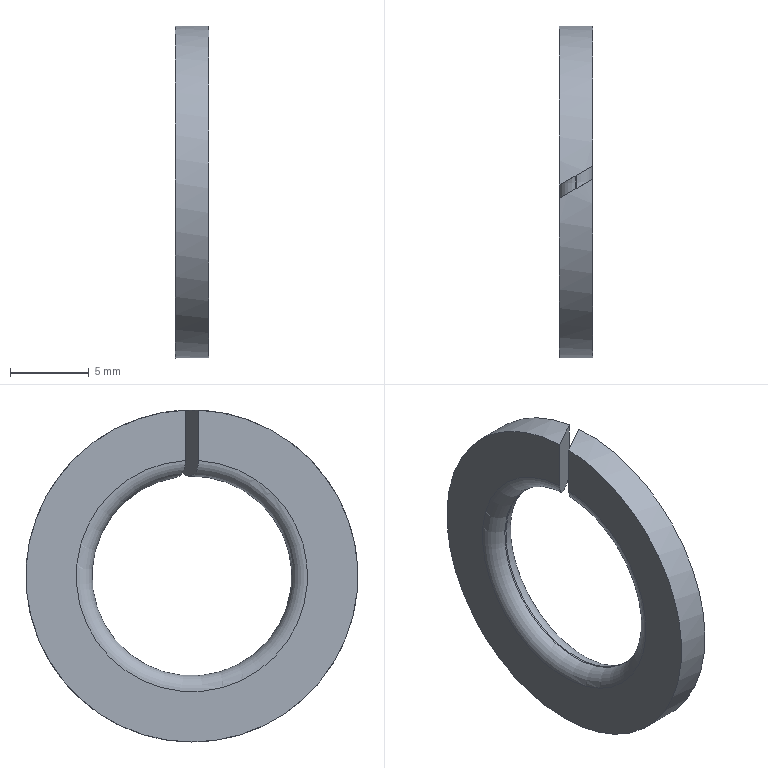Part | STEP file | DIN 128 - A12 | 1 solid | 8 faces | box 2.1 x 21.1 x 21.1 mm | volume 443.477 mm3 | plane 4 | cylinder 2 | torus 2 | commonest cylinder face diameters 12.7 x1 21.1 x1
STEP:
#1=CARTESIAN_POINT('',(0.,0.,0.));
#2=DIRECTION('',(0.,0.,1.));
#3=DIRECTION('',(1.,0.,0.));
#4=AXIS2_PLACEMENT_3D('',#1,#2,#3);
#5=CARTESIAN_POINT('',(2.1,1.632,7.166));
#6=VERTEX_POINT('',#5);
#7=CARTESIAN_POINT('',(1.1,1.055,6.262));
#8=VERTEX_POINT('',#7);
#9=CARTESIAN_POINT('',(2.1,1.632,7.166));
#10=CARTESIAN_POINT('',(2.1,1.632,7.046));
#11=CARTESIAN_POINT('',(2.074,1.617,6.906));
#12=CARTESIAN_POINT('',(1.985,1.566,6.688));
#13=CARTESIAN_POINT('',(1.907,1.521,6.575));
#14=CARTESIAN_POINT('',(1.739,1.424,6.415));
#15=CARTESIAN_POINT('',(1.618,1.354,6.344));
#16=CARTESIAN_POINT('',(1.385,1.219,6.264));
#17=CARTESIAN_POINT('',(1.229,1.13,6.249));
#18=CARTESIAN_POINT('',(1.1,1.055,6.262));
#19=B_SPLINE_CURVE_WITH_KNOTS('',3,(#9,#10,#11,#12,#13,#14,#15,#16,#17,#18),.UNSPECIFIED.,.F.,.F.,(4,2,2,2,4),(0.1661,0.2021,0.2382,0.2775,0.3225),.UNSPECIFIED.);
#20=CARTESIAN_POINT('',(0.,0.42,0.));
#21=DIRECTION('',(-0.5,0.866,0.));
#22=DIRECTION('',(0.,0.,1.));
#23=AXIS2_PLACEMENT_3D('',#20,#21,#22);
#24=PLANE('',#23);
#25=CARTESIAN_POINT('',(7.166,2.425));
#26=CARTESIAN_POINT('',(7.046,2.425));
#27=CARTESIAN_POINT('',(6.906,2.394));
#28=CARTESIAN_POINT('',(6.688,2.292));
#29=CARTESIAN_POINT('',(6.575,2.202));
#30=CARTESIAN_POINT('',(6.415,2.009));
#31=CARTESIAN_POINT('',(6.344,1.868));
#32=CARTESIAN_POINT('',(6.264,1.599));
#33=CARTESIAN_POINT('',(6.249,1.42));
#34=CARTESIAN_POINT('',(6.262,1.27));
#35=B_SPLINE_CURVE_WITH_KNOTS('',3,(#25,#26,#27,#28,#29,#30,#31,#32,#33,#34),.UNSPECIFIED.,.F.,.F.,(4,2,2,2,4),(0.1661,0.2021,0.2382,0.2775,0.3225),.UNSPECIFIED.);
#36=(GEOMETRIC_REPRESENTATION_CONTEXT(2)PARAMETRIC_REPRESENTATION_CONTEXT()REPRESENTATION_CONTEXT('',''));
#37=DEFINITIONAL_REPRESENTATION('',(#35),#36);
#38=PCURVE('',#24,#37);
#39=CARTESIAN_POINT('',(1.1,0.,0.));
#40=DIRECTION('',(-1.,0.,0.));
#41=DIRECTION('',(0.,0.,1.));
#42=AXIS2_PLACEMENT_3D('',#39,#40,#41);
#43=TOROIDAL_SURFACE('',#42,7.35,1.);
#44=CARTESIAN_POINT('',(0.224,4.712));
#45=CARTESIAN_POINT('',(0.2247,4.689));
#46=CARTESIAN_POINT('',(0.226,4.641));
#47=CARTESIAN_POINT('',(0.2277,4.566));
#48=CARTESIAN_POINT('',(0.229,4.488));
#49=CARTESIAN_POINT('',(0.2298,4.412));
#50=CARTESIAN_POINT('',(0.2301,4.339));
#51=CARTESIAN_POINT('',(0.2299,4.267));
#52=CARTESIAN_POINT('',(0.229,4.19));
#53=CARTESIAN_POINT('',(0.2277,4.113));
#54=CARTESIAN_POINT('',(0.2259,4.037));
#55=CARTESIAN_POINT('',(0.2236,3.965));
#56=CARTESIAN_POINT('',(0.2209,3.896));
#57=CARTESIAN_POINT('',(0.2175,3.823));
#58=CARTESIAN_POINT('',(0.2137,3.75));
#59=CARTESIAN_POINT('',(0.2095,3.677));
#60=CARTESIAN_POINT('',(0.205,3.607));
#61=CARTESIAN_POINT('',(0.2005,3.542));
#62=CARTESIAN_POINT('',(0.1955,3.476));
#63=CARTESIAN_POINT('',(0.1901,3.407));
#64=CARTESIAN_POINT('',(0.1844,3.338));
#65=CARTESIAN_POINT('',(0.1785,3.27));
#66=CARTESIAN_POINT('',(0.1727,3.204));
#67=CARTESIAN_POINT('',(0.1688,3.162));
#68=CARTESIAN_POINT('',(0.1669,3.142));
#69=B_SPLINE_CURVE_WITH_KNOTS('',3,(#44,#45,#46,#47,#48,#49,#50,#51,#52,#53,#54,#55,#56,#57,#58,#59,#60,#61,#62,#63,#64,#65,#66,#67,#68),.UNSPECIFIED.,.F.,.F.,(4,1,1,1,1,1,1,1,1,1,1,1,1,1,1,1,1,1,1,1,1,1,4),(0.1661,0.1732,0.1803,0.1874,0.1945,0.2016,0.2087,0.2158,0.2229,0.2301,0.2372,0.2443,0.2514,0.2585,0.2656,0.2727,0.2798,0.2869,0.294,0.3011,0.3083,0.3154,0.3225),.QUASI_UNIFORM_KNOTS.);
#70=(GEOMETRIC_REPRESENTATION_CONTEXT(2)PARAMETRIC_REPRESENTATION_CONTEXT()REPRESENTATION_CONTEXT('',''));
#71=DEFINITIONAL_REPRESENTATION('',(#69),#70);
#72=PCURVE('',#43,#71);
#73=SURFACE_CURVE('',#19,(#38,#72),.PCURVE_S1.);
#74=EDGE_CURVE('',#6,#8,#73,.T.);
#75=ORIENTED_EDGE('',*,*,#74,.F.);
#76=CARTESIAN_POINT('',(2.1,1.632,10.423));
#77=VERTEX_POINT('',#76);
#78=CARTESIAN_POINT('',(2.1,1.632,0.));
#79=DIRECTION('',(0.,0.,-1.));
#80=VECTOR('',#79,1.);
#81=LINE('',#78,#80);
#82=CARTESIAN_POINT('',(0.,2.425));
#83=DIRECTION('',(-1.,0.));
#84=VECTOR('',#83,1.);
#85=LINE('',#82,#84);
#86=(GEOMETRIC_REPRESENTATION_CONTEXT(2)PARAMETRIC_REPRESENTATION_CONTEXT()REPRESENTATION_CONTEXT('',''));
#87=DEFINITIONAL_REPRESENTATION('',(#85),#86);
#88=PCURVE('',#24,#87);
#89=CARTESIAN_POINT('',(2.1,0.,0.));
#90=DIRECTION('',(-1.,0.,0.));
#91=DIRECTION('',(0.,0.,1.));
#92=AXIS2_PLACEMENT_3D('',#89,#90,#91);
#93=PLANE('',#92);
#94=CARTESIAN_POINT('',(0.,1.632));
#95=DIRECTION('',(-1.,0.));
#96=VECTOR('',#95,1.);
#97=LINE('',#94,#96);
#98=(GEOMETRIC_REPRESENTATION_CONTEXT(2)PARAMETRIC_REPRESENTATION_CONTEXT()REPRESENTATION_CONTEXT('',''));
#99=DEFINITIONAL_REPRESENTATION('',(#97),#98);
#100=PCURVE('',#93,#99);
#101=SURFACE_CURVE('',#81,(#88,#100),.PCURVE_S1.);
#102=EDGE_CURVE('',#77,#6,#101,.T.);
#103=ORIENTED_EDGE('',*,*,#102,.F.);
#104=CARTESIAN_POINT('',(0.,0.42,10.542));
#105=VERTEX_POINT('',#104);
#106=CARTESIAN_POINT('',(-0.7275,0.,0.));
#107=DIRECTION('',(-0.5,0.866,0.));
#108=DIRECTION('',(-0.866,-0.5,0.));
#109=AXIS2_PLACEMENT_3D('',#106,#107,#108);
#110=ELLIPSE('',#109,21.1,10.55);
#111=CARTESIAN_POINT('',(0.,-0.84));
#112=DIRECTION('',(0.,-1.));
#113=AXIS2_PLACEMENT_2D('',#111,#112);
#114=ELLIPSE('',#113,21.1,10.55);
#115=(GEOMETRIC_REPRESENTATION_CONTEXT(2)PARAMETRIC_REPRESENTATION_CONTEXT()REPRESENTATION_CONTEXT('',''));
#116=DEFINITIONAL_REPRESENTATION('',(#114),#115);
#117=PCURVE('',#24,#116);
#118=CARTESIAN_POINT('',(0.,0.,0.));
#119=DIRECTION('',(1.,0.,0.));
#120=DIRECTION('',(0.,-1.,0.));
#121=AXIS2_PLACEMENT_3D('',#118,#119,#120);
#122=CYLINDRICAL_SURFACE('',#121,10.55);
#123=CARTESIAN_POINT('',(4.673,0.));
#124=CARTESIAN_POINT('',(4.557,2.1));
#125=B_SPLINE_CURVE_WITH_KNOTS('',1,(#123,#124),.UNSPECIFIED.,.F.,.F.,(2,2),(1.611,1.726),.PIECEWISE_BEZIER_KNOTS.);
#126=(GEOMETRIC_REPRESENTATION_CONTEXT(2)PARAMETRIC_REPRESENTATION_CONTEXT()REPRESENTATION_CONTEXT('',''));
#127=DEFINITIONAL_REPRESENTATION('',(#125),#126);
#128=PCURVE('',#122,#127);
#129=SURFACE_CURVE('',#110,(#117,#128),.PCURVE_S1.);
#130=EDGE_CURVE('',#105,#77,#129,.T.);
#131=ORIENTED_EDGE('',*,*,#130,.F.);
#132=CARTESIAN_POINT('',(0.,0.42,7.338));
#133=VERTEX_POINT('',#132);
#134=CARTESIAN_POINT('',(0.,0.42,0.));
#135=DIRECTION('',(0.,0.,1.));
#136=VECTOR('',#135,1.);
#137=LINE('',#134,#136);
#138=CARTESIAN_POINT('',(0.,0.));
#139=DIRECTION('',(1.,0.));
#140=VECTOR('',#139,1.);
#141=LINE('',#138,#140);
#142=(GEOMETRIC_REPRESENTATION_CONTEXT(2)PARAMETRIC_REPRESENTATION_CONTEXT()REPRESENTATION_CONTEXT('',''));
#143=DEFINITIONAL_REPRESENTATION('',(#141),#142);
#144=PCURVE('',#24,#143);
#145=CARTESIAN_POINT('',(0.,0.,0.));
#146=DIRECTION('',(-1.,0.,0.));
#147=DIRECTION('',(0.,0.,1.));
#148=AXIS2_PLACEMENT_3D('',#145,#146,#147);
#149=PLANE('',#148);
#150=CARTESIAN_POINT('',(0.,0.42));
#151=DIRECTION('',(1.,0.));
#152=VECTOR('',#151,1.);
#153=LINE('',#150,#152);
#154=(GEOMETRIC_REPRESENTATION_CONTEXT(2)PARAMETRIC_REPRESENTATION_CONTEXT()REPRESENTATION_CONTEXT('',''));
#155=DEFINITIONAL_REPRESENTATION('',(#153),#154);
#156=PCURVE('',#149,#155);
#157=SURFACE_CURVE('',#137,(#144,#156),.PCURVE_S1.);
#158=EDGE_CURVE('',#133,#105,#157,.T.);
#159=ORIENTED_EDGE('',*,*,#158,.F.);
#160=CARTESIAN_POINT('',(1.,0.9974,6.271));
#161=VERTEX_POINT('',#160);
#162=CARTESIAN_POINT('',(1.,0.9974,6.271));
#163=CARTESIAN_POINT('',(0.869,0.9217,6.283));
#164=CARTESIAN_POINT('',(0.7161,0.8334,6.328));
#165=CARTESIAN_POINT('',(0.4826,0.6987,6.448));
#166=CARTESIAN_POINT('',(0.3583,0.6269,6.542));
#167=CARTESIAN_POINT('',(0.1893,0.5293,6.732));
#168=CARTESIAN_POINT('',(0.1111,0.4841,6.858));
#169=CARTESIAN_POINT('',(0.02592,0.435,7.084));
#170=CARTESIAN_POINT('',(0.,0.42,7.221));
#171=CARTESIAN_POINT('',(0.,0.42,7.338));
#172=B_SPLINE_CURVE_WITH_KNOTS('',3,(#162,#163,#164,#165,#166,#167,#168,#169,#170,#171),.UNSPECIFIED.,.F.,.F.,(4,2,2,2,4),(0.3222,0.3678,0.4107,0.4495,0.4845),.UNSPECIFIED.);
#173=CARTESIAN_POINT('',(6.271,1.155));
#174=CARTESIAN_POINT('',(6.283,1.003));
#175=CARTESIAN_POINT('',(6.328,0.8268));
#176=CARTESIAN_POINT('',(6.448,0.5573));
#177=CARTESIAN_POINT('',(6.542,0.4137));
#178=CARTESIAN_POINT('',(6.732,0.2186));
#179=CARTESIAN_POINT('',(6.858,0.1283));
#180=CARTESIAN_POINT('',(7.084,0.02993));
#181=CARTESIAN_POINT('',(7.221,0.));
#182=CARTESIAN_POINT('',(7.338,0.));
#183=B_SPLINE_CURVE_WITH_KNOTS('',3,(#173,#174,#175,#176,#177,#178,#179,#180,#181,#182),.UNSPECIFIED.,.F.,.F.,(4,2,2,2,4),(0.3222,0.3678,0.4107,0.4495,0.4845),.UNSPECIFIED.);
#184=(GEOMETRIC_REPRESENTATION_CONTEXT(2)PARAMETRIC_REPRESENTATION_CONTEXT()REPRESENTATION_CONTEXT('',''));
#185=DEFINITIONAL_REPRESENTATION('',(#183),#184);
#186=PCURVE('',#24,#185);
#187=CARTESIAN_POINT('',(1.,0.,0.));
#188=DIRECTION('',(1.,0.,0.));
#189=DIRECTION('',(0.,0.,-1.));
#190=AXIS2_PLACEMENT_3D('',#187,#188,#189);
#191=TOROIDAL_SURFACE('',#190,7.35,1.);
#192=CARTESIAN_POINT('',(9.267,3.142));
#193=CARTESIAN_POINT('',(9.269,3.163));
#194=CARTESIAN_POINT('',(9.273,3.206));
#195=CARTESIAN_POINT('',(9.279,3.274));
#196=CARTESIAN_POINT('',(9.286,3.343));
#197=CARTESIAN_POINT('',(9.292,3.413));
#198=CARTESIAN_POINT('',(9.299,3.481));
#199=CARTESIAN_POINT('',(9.305,3.547));
#200=CARTESIAN_POINT('',(9.311,3.611));
#201=CARTESIAN_POINT('',(9.317,3.68));
#202=CARTESIAN_POINT('',(9.322,3.751));
#203=CARTESIAN_POINT('',(9.328,3.822));
#204=CARTESIAN_POINT('',(9.334,3.893));
#205=CARTESIAN_POINT('',(9.338,3.961));
#206=CARTESIAN_POINT('',(9.343,4.03));
#207=CARTESIAN_POINT('',(9.347,4.104));
#208=CARTESIAN_POINT('',(9.352,4.179));
#209=CARTESIAN_POINT('',(9.355,4.255));
#210=CARTESIAN_POINT('',(9.359,4.329));
#211=CARTESIAN_POINT('',(9.361,4.4));
#212=CARTESIAN_POINT('',(9.364,4.478));
#213=CARTESIAN_POINT('',(9.365,4.558));
#214=CARTESIAN_POINT('',(9.367,4.637));
#215=CARTESIAN_POINT('',(9.367,4.688));
#216=CARTESIAN_POINT('',(9.368,4.712));
#217=B_SPLINE_CURVE_WITH_KNOTS('',3,(#192,#193,#194,#195,#196,#197,#198,#199,#200,#201,#202,#203,#204,#205,#206,#207,#208,#209,#210,#211,#212,#213,#214,#215,#216),.UNSPECIFIED.,.F.,.F.,(4,1,1,1,1,1,1,1,1,1,1,1,1,1,1,1,1,1,1,1,1,1,4),(0.3222,0.3296,0.337,0.3444,0.3517,0.3591,0.3665,0.3739,0.3812,0.3886,0.396,0.4034,0.4108,0.4181,0.4255,0.4329,0.4403,0.4477,0.455,0.4624,0.4698,0.4772,0.4845),.QUASI_UNIFORM_KNOTS.);
#218=(GEOMETRIC_REPRESENTATION_CONTEXT(2)PARAMETRIC_REPRESENTATION_CONTEXT()REPRESENTATION_CONTEXT('',''));
#219=DEFINITIONAL_REPRESENTATION('',(#217),#218);
#220=PCURVE('',#191,#219);
#221=SURFACE_CURVE('',#172,(#186,#220),.PCURVE_S1.);
#222=EDGE_CURVE('',#161,#133,#221,.T.);
#223=ORIENTED_EDGE('',*,*,#222,.F.);
#224=CARTESIAN_POINT('',(-0.7275,0.,0.));
#225=DIRECTION('',(0.5,-0.866,0.));
#226=DIRECTION('',(-0.866,-0.5,0.));
#227=AXIS2_PLACEMENT_3D('',#224,#225,#226);
#228=ELLIPSE('',#227,12.7,6.35);
#229=CARTESIAN_POINT('',(0.,-13.54));
#230=CARTESIAN_POINT('',(-10.999,-13.54));
#231=CARTESIAN_POINT('',(-5.499,5.51));
#232=CARTESIAN_POINT('',(0.,24.56));
#233=CARTESIAN_POINT('',(5.499,5.51));
#234=CARTESIAN_POINT('',(10.999,-13.54));
#235=CARTESIAN_POINT('',(0.,-13.54));
#236=(BOUNDED_CURVE()B_SPLINE_CURVE(2,(#229,#230,#231,#232,#233,#234,#235),.UNSPECIFIED.,.T.,.F.)B_SPLINE_CURVE_WITH_KNOTS((1,2,2,2,2,1),(-2.094,0.,2.094,4.189,6.283,8.378),.UNSPECIFIED.)CURVE()GEOMETRIC_REPRESENTATION_ITEM()RATIONAL_B_SPLINE_CURVE((1.,0.5,1.,0.5,1.,0.5,1.))REPRESENTATION_ITEM(''));
#237=(GEOMETRIC_REPRESENTATION_CONTEXT(2)PARAMETRIC_REPRESENTATION_CONTEXT()REPRESENTATION_CONTEXT('',''));
#238=DEFINITIONAL_REPRESENTATION('',(#236),#237);
#239=PCURVE('',#24,#238);
#240=CARTESIAN_POINT('',(0.,0.,0.));
#241=DIRECTION('',(1.,0.,0.));
#242=DIRECTION('',(0.,-1.,0.));
#243=AXIS2_PLACEMENT_3D('',#240,#241,#242);
#244=CYLINDRICAL_SURFACE('',#243,6.35);
#245=CARTESIAN_POINT('',(4.545,1.1));
#246=CARTESIAN_POINT('',(4.555,1.));
#247=B_SPLINE_CURVE_WITH_KNOTS('',1,(#245,#246),.UNSPECIFIED.,.F.,.F.,(2,2),(4.545,4.555),.PIECEWISE_BEZIER_KNOTS.);
#248=(GEOMETRIC_REPRESENTATION_CONTEXT(2)PARAMETRIC_REPRESENTATION_CONTEXT()REPRESENTATION_CONTEXT('',''));
#249=DEFINITIONAL_REPRESENTATION('',(#247),#248);
#250=PCURVE('',#244,#249);
#251=SURFACE_CURVE('',#228,(#239,#250),.PCURVE_S1.);
#252=EDGE_CURVE('',#8,#161,#251,.T.);
#253=ORIENTED_EDGE('',*,*,#252,.F.);
#254=EDGE_LOOP('',(#75,#103,#131,#159,#223,#253));
#255=FACE_BOUND('',#254,.T.);
#256=ADVANCED_FACE('',(#255),#24,.F.);
#257=CARTESIAN_POINT('',(1.1,0.2151,6.346));
#258=VERTEX_POINT('',#257);
#259=CARTESIAN_POINT('',(2.1,0.7924,7.307));
#260=VERTEX_POINT('',#259);
#261=CARTESIAN_POINT('',(1.1,0.2151,6.346));
#262=CARTESIAN_POINT('',(1.23,0.2903,6.344));
#263=CARTESIAN_POINT('',(1.385,0.3796,6.371));
#264=CARTESIAN_POINT('',(1.619,0.5145,6.466));
#265=CARTESIAN_POINT('',(1.741,0.5853,6.546));
#266=CARTESIAN_POINT('',(1.909,0.6824,6.717));
#267=CARTESIAN_POINT('',(1.987,0.7272,6.834));
#268=CARTESIAN_POINT('',(2.074,0.7774,7.052));
#269=CARTESIAN_POINT('',(2.1,0.7924,7.19));
#270=CARTESIAN_POINT('',(2.1,0.7924,7.307));
#271=B_SPLINE_CURVE_WITH_KNOTS('',3,(#261,#262,#263,#264,#265,#266,#267,#268,#269,#270),.UNSPECIFIED.,.F.,.F.,(4,2,2,2,4),(0.3195,0.3647,0.4054,0.4422,0.4774),.UNSPECIFIED.);
#272=CARTESIAN_POINT('',(2.1,0.7924,0.));
#273=DIRECTION('',(0.5,-0.866,0.));
#274=DIRECTION('',(0.,0.,-1.));
#275=AXIS2_PLACEMENT_3D('',#272,#273,#274);
#276=PLANE('',#275);
#277=CARTESIAN_POINT('',(-6.346,-1.155));
#278=CARTESIAN_POINT('',(-6.344,-1.004));
#279=CARTESIAN_POINT('',(-6.371,-0.8256));
#280=CARTESIAN_POINT('',(-6.466,-0.5559));
#281=CARTESIAN_POINT('',(-6.546,-0.4142));
#282=CARTESIAN_POINT('',(-6.717,-0.2201));
#283=CARTESIAN_POINT('',(-6.834,-0.1304));
#284=CARTESIAN_POINT('',(-7.052,-0.03008));
#285=CARTESIAN_POINT('',(-7.19,0.));
#286=CARTESIAN_POINT('',(-7.307,0.));
#287=B_SPLINE_CURVE_WITH_KNOTS('',3,(#277,#278,#279,#280,#281,#282,#283,#284,#285,#286),.UNSPECIFIED.,.F.,.F.,(4,2,2,2,4),(0.3195,0.3647,0.4054,0.4422,0.4774),.UNSPECIFIED.);
#288=(GEOMETRIC_REPRESENTATION_CONTEXT(2)PARAMETRIC_REPRESENTATION_CONTEXT()REPRESENTATION_CONTEXT('',''));
#289=DEFINITIONAL_REPRESENTATION('',(#287),#288);
#290=PCURVE('',#276,#289);
#291=CARTESIAN_POINT('',(6.317,3.142));
#292=CARTESIAN_POINT('',(6.319,3.162));
#293=CARTESIAN_POINT('',(6.323,3.205));
#294=CARTESIAN_POINT('',(6.329,3.272));
#295=CARTESIAN_POINT('',(6.335,3.34));
#296=CARTESIAN_POINT('',(6.341,3.409));
#297=CARTESIAN_POINT('',(6.346,3.477));
#298=CARTESIAN_POINT('',(6.352,3.543));
#299=CARTESIAN_POINT('',(6.357,3.607));
#300=CARTESIAN_POINT('',(6.362,3.677));
#301=CARTESIAN_POINT('',(6.367,3.749));
#302=CARTESIAN_POINT('',(6.371,3.821));
#303=CARTESIAN_POINT('',(6.375,3.893));
#304=CARTESIAN_POINT('',(6.379,3.962));
#305=CARTESIAN_POINT('',(6.382,4.032));
#306=CARTESIAN_POINT('',(6.385,4.107));
#307=CARTESIAN_POINT('',(6.388,4.184));
#308=CARTESIAN_POINT('',(6.39,4.26));
#309=CARTESIAN_POINT('',(6.391,4.333));
#310=CARTESIAN_POINT('',(6.392,4.406));
#311=CARTESIAN_POINT('',(6.393,4.483));
#312=CARTESIAN_POINT('',(6.393,4.562));
#313=CARTESIAN_POINT('',(6.392,4.639));
#314=CARTESIAN_POINT('',(6.392,4.689));
#315=CARTESIAN_POINT('',(6.391,4.712));
#316=B_SPLINE_CURVE_WITH_KNOTS('',3,(#291,#292,#293,#294,#295,#296,#297,#298,#299,#300,#301,#302,#303,#304,#305,#306,#307,#308,#309,#310,#311,#312,#313,#314,#315),.UNSPECIFIED.,.F.,.F.,(4,1,1,1,1,1,1,1,1,1,1,1,1,1,1,1,1,1,1,1,1,1,4),(0.3195,0.3267,0.3339,0.3411,0.3483,0.3554,0.3626,0.3698,0.377,0.3841,0.3913,0.3985,0.4057,0.4129,0.42,0.4272,0.4344,0.4416,0.4487,0.4559,0.4631,0.4703,0.4774),.QUASI_UNIFORM_KNOTS.);
#317=(GEOMETRIC_REPRESENTATION_CONTEXT(2)PARAMETRIC_REPRESENTATION_CONTEXT()REPRESENTATION_CONTEXT('',''));
#318=DEFINITIONAL_REPRESENTATION('',(#316),#317);
#319=PCURVE('',#43,#318);
#320=SURFACE_CURVE('',#271,(#290,#319),.PCURVE_S1.);
#321=EDGE_CURVE('',#258,#260,#320,.T.);
#322=ORIENTED_EDGE('',*,*,#321,.F.);
#323=CARTESIAN_POINT('',(1.,0.1574,6.348));
#324=VERTEX_POINT('',#323);
#325=CARTESIAN_POINT('',(0.7275,0.,0.));
#326=DIRECTION('',(-0.5,0.866,0.));
#327=DIRECTION('',(-0.866,-0.5,0.));
#328=AXIS2_PLACEMENT_3D('',#325,#326,#327);
#329=ELLIPSE('',#328,12.7,6.35);
#330=CARTESIAN_POINT('',(0.,-14.285));
#331=CARTESIAN_POINT('',(-10.999,-14.285));
#332=CARTESIAN_POINT('',(-5.499,4.765));
#333=CARTESIAN_POINT('',(0.,23.815));
#334=CARTESIAN_POINT('',(5.499,4.765));
#335=CARTESIAN_POINT('',(10.999,-14.285));
#336=CARTESIAN_POINT('',(0.,-14.285));
#337=(BOUNDED_CURVE()B_SPLINE_CURVE(2,(#330,#331,#332,#333,#334,#335,#336),.UNSPECIFIED.,.T.,.F.)B_SPLINE_CURVE_WITH_KNOTS((1,2,2,2,2,1),(-2.094,0.,2.094,4.189,6.283,8.378),.UNSPECIFIED.)CURVE()GEOMETRIC_REPRESENTATION_ITEM()RATIONAL_B_SPLINE_CURVE((1.,0.5,1.,0.5,1.,0.5,1.))REPRESENTATION_ITEM(''));
#338=(GEOMETRIC_REPRESENTATION_CONTEXT(2)PARAMETRIC_REPRESENTATION_CONTEXT()REPRESENTATION_CONTEXT('',''));
#339=DEFINITIONAL_REPRESENTATION('',(#337),#338);
#340=PCURVE('',#276,#339);
#341=CARTESIAN_POINT('',(-1.596,1.));
#342=CARTESIAN_POINT('',(-1.605,1.1));
#343=B_SPLINE_CURVE_WITH_KNOTS('',1,(#341,#342),.UNSPECIFIED.,.F.,.F.,(2,2),(1.596,1.605),.PIECEWISE_BEZIER_KNOTS.);
#344=(GEOMETRIC_REPRESENTATION_CONTEXT(2)PARAMETRIC_REPRESENTATION_CONTEXT()REPRESENTATION_CONTEXT('',''));
#345=DEFINITIONAL_REPRESENTATION('',(#343),#344);
#346=PCURVE('',#244,#345);
#347=SURFACE_CURVE('',#329,(#340,#346),.PCURVE_S1.);
#348=EDGE_CURVE('',#324,#258,#347,.T.);
#349=ORIENTED_EDGE('',*,*,#348,.F.);
#350=CARTESIAN_POINT('',(0.,-0.42,7.338));
#351=VERTEX_POINT('',#350);
#352=CARTESIAN_POINT('',(0.,-0.42,7.338));
#353=CARTESIAN_POINT('',(0.,-0.42,7.221));
#354=CARTESIAN_POINT('',(0.02598,-0.405,7.084));
#355=CARTESIAN_POINT('',(0.1122,-0.3552,6.864));
#356=CARTESIAN_POINT('',(0.19,-0.3103,6.745));
#357=CARTESIAN_POINT('',(0.3583,-0.2131,6.569));
#358=CARTESIAN_POINT('',(0.4815,-0.142,6.485));
#359=CARTESIAN_POINT('',(0.7151,-0.007115,6.383));
#360=CARTESIAN_POINT('',(0.8694,0.08192,6.35));
#361=CARTESIAN_POINT('',(1.,0.1574,6.348));
#362=B_SPLINE_CURVE_WITH_KNOTS('',3,(#352,#353,#354,#355,#356,#357,#358,#359,#360,#361),.UNSPECIFIED.,.F.,.F.,(4,2,2,2,4),(0.1606,0.1956,0.233,0.2743,0.3196),.UNSPECIFIED.);
#363=CARTESIAN_POINT('',(-7.338,-2.425));
#364=CARTESIAN_POINT('',(-7.221,-2.425));
#365=CARTESIAN_POINT('',(-7.084,-2.395));
#366=CARTESIAN_POINT('',(-6.864,-2.295));
#367=CARTESIAN_POINT('',(-6.745,-2.205));
#368=CARTESIAN_POINT('',(-6.569,-2.011));
#369=CARTESIAN_POINT('',(-6.485,-1.869));
#370=CARTESIAN_POINT('',(-6.383,-1.599));
#371=CARTESIAN_POINT('',(-6.35,-1.421));
#372=CARTESIAN_POINT('',(-6.348,-1.27));
#373=B_SPLINE_CURVE_WITH_KNOTS('',3,(#363,#364,#365,#366,#367,#368,#369,#370,#371,#372),.UNSPECIFIED.,.F.,.F.,(4,2,2,2,4),(0.1606,0.1956,0.233,0.2743,0.3196),.UNSPECIFIED.);
#374=(GEOMETRIC_REPRESENTATION_CONTEXT(2)PARAMETRIC_REPRESENTATION_CONTEXT()REPRESENTATION_CONTEXT('',''));
#375=DEFINITIONAL_REPRESENTATION('',(#373),#374);
#376=PCURVE('',#276,#375);
#377=CARTESIAN_POINT('',(3.199,4.712));
#378=CARTESIAN_POINT('',(3.199,4.688));
#379=CARTESIAN_POINT('',(3.199,4.638));
#380=CARTESIAN_POINT('',(3.199,4.56));
#381=CARTESIAN_POINT('',(3.198,4.482));
#382=CARTESIAN_POINT('',(3.197,4.404));
#383=CARTESIAN_POINT('',(3.196,4.332));
#384=CARTESIAN_POINT('',(3.194,4.258));
#385=CARTESIAN_POINT('',(3.191,4.182));
#386=CARTESIAN_POINT('',(3.188,4.106));
#387=CARTESIAN_POINT('',(3.185,4.031));
#388=CARTESIAN_POINT('',(3.181,3.961));
#389=CARTESIAN_POINT('',(3.177,3.893));
#390=CARTESIAN_POINT('',(3.173,3.821));
#391=CARTESIAN_POINT('',(3.168,3.749));
#392=CARTESIAN_POINT('',(3.163,3.678));
#393=CARTESIAN_POINT('',(3.157,3.608));
#394=CARTESIAN_POINT('',(3.152,3.544));
#395=CARTESIAN_POINT('',(3.147,3.478));
#396=CARTESIAN_POINT('',(3.141,3.41));
#397=CARTESIAN_POINT('',(3.135,3.341));
#398=CARTESIAN_POINT('',(3.129,3.272));
#399=CARTESIAN_POINT('',(3.123,3.205));
#400=CARTESIAN_POINT('',(3.119,3.162));
#401=CARTESIAN_POINT('',(3.117,3.142));
#402=B_SPLINE_CURVE_WITH_KNOTS('',3,(#377,#378,#379,#380,#381,#382,#383,#384,#385,#386,#387,#388,#389,#390,#391,#392,#393,#394,#395,#396,#397,#398,#399,#400,#401),.UNSPECIFIED.,.F.,.F.,(4,1,1,1,1,1,1,1,1,1,1,1,1,1,1,1,1,1,1,1,1,1,4),(0.1606,0.1678,0.175,0.1823,0.1895,0.1967,0.2039,0.2112,0.2184,0.2256,0.2329,0.2401,0.2473,0.2545,0.2618,0.269,0.2762,0.2834,0.2907,0.2979,0.3051,0.3123,0.3196),.QUASI_UNIFORM_KNOTS.);
#403=(GEOMETRIC_REPRESENTATION_CONTEXT(2)PARAMETRIC_REPRESENTATION_CONTEXT()REPRESENTATION_CONTEXT('',''));
#404=DEFINITIONAL_REPRESENTATION('',(#402),#403);
#405=PCURVE('',#191,#404);
#406=SURFACE_CURVE('',#362,(#376,#405),.PCURVE_S1.);
#407=EDGE_CURVE('',#351,#324,#406,.T.);
#408=ORIENTED_EDGE('',*,*,#407,.F.);
#409=CARTESIAN_POINT('',(0.,-0.42,10.542));
#410=VERTEX_POINT('',#409);
#411=CARTESIAN_POINT('',(0.,-0.42,0.));
#412=DIRECTION('',(0.,0.,-1.));
#413=VECTOR('',#412,1.);
#414=LINE('',#411,#413);
#415=CARTESIAN_POINT('',(0.,-2.425));
#416=DIRECTION('',(1.,0.));
#417=VECTOR('',#416,1.);
#418=LINE('',#415,#417);
#419=(GEOMETRIC_REPRESENTATION_CONTEXT(2)PARAMETRIC_REPRESENTATION_CONTEXT()REPRESENTATION_CONTEXT('',''));
#420=DEFINITIONAL_REPRESENTATION('',(#418),#419);
#421=PCURVE('',#276,#420);
#422=CARTESIAN_POINT('',(0.,-0.42));
#423=DIRECTION('',(-1.,0.));
#424=VECTOR('',#423,1.);
#425=LINE('',#422,#424);
#426=(GEOMETRIC_REPRESENTATION_CONTEXT(2)PARAMETRIC_REPRESENTATION_CONTEXT()REPRESENTATION_CONTEXT('',''));
#427=DEFINITIONAL_REPRESENTATION('',(#425),#426);
#428=PCURVE('',#149,#427);
#429=SURFACE_CURVE('',#414,(#421,#428),.PCURVE_S1.);
#430=EDGE_CURVE('',#410,#351,#429,.T.);
#431=ORIENTED_EDGE('',*,*,#430,.F.);
#432=CARTESIAN_POINT('',(2.1,0.7924,10.52));
#433=VERTEX_POINT('',#432);
#434=CARTESIAN_POINT('',(0.7275,0.,0.));
#435=DIRECTION('',(0.5,-0.866,0.));
#436=DIRECTION('',(-0.866,-0.5,0.));
#437=AXIS2_PLACEMENT_3D('',#434,#435,#436);
#438=ELLIPSE('',#437,21.1,10.55);
#439=CARTESIAN_POINT('',(0.,-1.585));
#440=DIRECTION('',(0.,-1.));
#441=AXIS2_PLACEMENT_2D('',#439,#440);
#442=ELLIPSE('',#441,21.1,10.55);
#443=(GEOMETRIC_REPRESENTATION_CONTEXT(2)PARAMETRIC_REPRESENTATION_CONTEXT()REPRESENTATION_CONTEXT('',''));
#444=DEFINITIONAL_REPRESENTATION('',(#442),#443);
#445=PCURVE('',#276,#444);
#446=CARTESIAN_POINT('',(-1.646,2.1));
#447=CARTESIAN_POINT('',(-1.531,0.));
#448=B_SPLINE_CURVE_WITH_KNOTS('',1,(#446,#447),.UNSPECIFIED.,.F.,.F.,(2,2),(4.637,4.752),.PIECEWISE_BEZIER_KNOTS.);
#449=(GEOMETRIC_REPRESENTATION_CONTEXT(2)PARAMETRIC_REPRESENTATION_CONTEXT()REPRESENTATION_CONTEXT('',''));
#450=DEFINITIONAL_REPRESENTATION('',(#448),#449);
#451=PCURVE('',#122,#450);
#452=SURFACE_CURVE('',#438,(#445,#451),.PCURVE_S1.);
#453=EDGE_CURVE('',#433,#410,#452,.T.);
#454=ORIENTED_EDGE('',*,*,#453,.F.);
#455=CARTESIAN_POINT('',(2.1,0.7924,0.));
#456=DIRECTION('',(0.,0.,1.));
#457=VECTOR('',#456,1.);
#458=LINE('',#455,#457);
#459=CARTESIAN_POINT('',(0.,0.));
#460=DIRECTION('',(-1.,0.));
#461=VECTOR('',#460,1.);
#462=LINE('',#459,#461);
#463=(GEOMETRIC_REPRESENTATION_CONTEXT(2)PARAMETRIC_REPRESENTATION_CONTEXT()REPRESENTATION_CONTEXT('',''));
#464=DEFINITIONAL_REPRESENTATION('',(#462),#463);
#465=PCURVE('',#276,#464);
#466=CARTESIAN_POINT('',(0.,0.7924));
#467=DIRECTION('',(1.,0.));
#468=VECTOR('',#467,1.);
#469=LINE('',#466,#468);
#470=(GEOMETRIC_REPRESENTATION_CONTEXT(2)PARAMETRIC_REPRESENTATION_CONTEXT()REPRESENTATION_CONTEXT('',''));
#471=DEFINITIONAL_REPRESENTATION('',(#469),#470);
#472=PCURVE('',#93,#471);
#473=SURFACE_CURVE('',#458,(#465,#472),.PCURVE_S1.);
#474=EDGE_CURVE('',#260,#433,#473,.T.);
#475=ORIENTED_EDGE('',*,*,#474,.F.);
#476=EDGE_LOOP('',(#322,#349,#408,#431,#454,#475));
#477=FACE_BOUND('',#476,.T.);
#478=ADVANCED_FACE('',(#477),#276,.F.);
#479=CARTESIAN_POINT('',(1.1,0.,0.));
#480=DIRECTION('',(-1.,0.,0.));
#481=DIRECTION('',(0.,-1.,0.));
#482=AXIS2_PLACEMENT_3D('',#479,#480,#481);
#483=CIRCLE('',#482,6.35);
#484=CARTESIAN_POINT('',(6.283,1.1));
#485=DIRECTION('',(-1.,0.));
#486=VECTOR('',#485,1.);
#487=LINE('',#484,#486);
#488=(GEOMETRIC_REPRESENTATION_CONTEXT(2)PARAMETRIC_REPRESENTATION_CONTEXT()REPRESENTATION_CONTEXT('',''));
#489=DEFINITIONAL_REPRESENTATION('',(#487),#488);
#490=PCURVE('',#244,#489);
#491=CARTESIAN_POINT('',(-1.571,3.142));
#492=DIRECTION('',(1.,0.));
#493=VECTOR('',#492,1.);
#494=LINE('',#491,#493);
#495=(GEOMETRIC_REPRESENTATION_CONTEXT(2)PARAMETRIC_REPRESENTATION_CONTEXT()REPRESENTATION_CONTEXT('',''));
#496=DEFINITIONAL_REPRESENTATION('',(#494),#495);
#497=PCURVE('',#43,#496);
#498=SURFACE_CURVE('',#483,(#490,#497),.PCURVE_S1.);
#499=EDGE_CURVE('',#8,#258,#498,.T.);
#500=ORIENTED_EDGE('',*,*,#499,.T.);
#501=ORIENTED_EDGE('',*,*,#348,.F.);
#502=CARTESIAN_POINT('',(1.,0.,0.));
#503=DIRECTION('',(1.,0.,0.));
#504=DIRECTION('',(0.,-1.,0.));
#505=AXIS2_PLACEMENT_3D('',#502,#503,#504);
#506=CIRCLE('',#505,6.35);
#507=CARTESIAN_POINT('',(-6.283,1.));
#508=DIRECTION('',(1.,0.));
#509=VECTOR('',#508,1.);
#510=LINE('',#507,#509);
#511=(GEOMETRIC_REPRESENTATION_CONTEXT(2)PARAMETRIC_REPRESENTATION_CONTEXT()REPRESENTATION_CONTEXT('',''));
#512=DEFINITIONAL_REPRESENTATION('',(#510),#511);
#513=PCURVE('',#244,#512);
#514=CARTESIAN_POINT('',(-1.571,3.142));
#515=DIRECTION('',(1.,0.));
#516=VECTOR('',#515,1.);
#517=LINE('',#514,#516);
#518=(GEOMETRIC_REPRESENTATION_CONTEXT(2)PARAMETRIC_REPRESENTATION_CONTEXT()REPRESENTATION_CONTEXT('',''));
#519=DEFINITIONAL_REPRESENTATION('',(#517),#518);
#520=PCURVE('',#191,#519);
#521=SURFACE_CURVE('',#506,(#513,#520),.PCURVE_S1.);
#522=EDGE_CURVE('',#324,#161,#521,.T.);
#523=ORIENTED_EDGE('',*,*,#522,.T.);
#524=ORIENTED_EDGE('',*,*,#252,.F.);
#525=EDGE_LOOP('',(#500,#501,#523,#524));
#526=FACE_BOUND('',#525,.F.);
#527=ADVANCED_FACE('',(#526),#244,.F.);
#528=ORIENTED_EDGE('',*,*,#222,.T.);
#529=CARTESIAN_POINT('',(0.,0.,0.));
#530=DIRECTION('',(-1.,0.,0.));
#531=DIRECTION('',(0.,-1.,0.));
#532=AXIS2_PLACEMENT_3D('',#529,#530,#531);
#533=CIRCLE('',#532,7.35);
#534=CARTESIAN_POINT('',(10.996,4.712));
#535=DIRECTION('',(-1.,0.));
#536=VECTOR('',#535,1.);
#537=LINE('',#534,#536);
#538=(GEOMETRIC_REPRESENTATION_CONTEXT(2)PARAMETRIC_REPRESENTATION_CONTEXT()REPRESENTATION_CONTEXT('',''));
#539=DEFINITIONAL_REPRESENTATION('',(#537),#538);
#540=PCURVE('',#191,#539);
#541=CARTESIAN_POINT('',(0.,0.));
#542=DIRECTION('',(0.,-1.));
#543=AXIS2_PLACEMENT_2D('',#541,#542);
#544=CIRCLE('',#543,7.35);
#545=(GEOMETRIC_REPRESENTATION_CONTEXT(2)PARAMETRIC_REPRESENTATION_CONTEXT()REPRESENTATION_CONTEXT('',''));
#546=DEFINITIONAL_REPRESENTATION('',(#544),#545);
#547=PCURVE('',#149,#546);
#548=SURFACE_CURVE('',#533,(#540,#547),.PCURVE_S1.);
#549=EDGE_CURVE('',#133,#351,#548,.T.);
#550=ORIENTED_EDGE('',*,*,#549,.T.);
#551=ORIENTED_EDGE('',*,*,#407,.T.);
#552=ORIENTED_EDGE('',*,*,#522,.T.);
#553=EDGE_LOOP('',(#528,#550,#551,#552));
#554=FACE_BOUND('',#553,.T.);
#555=ADVANCED_FACE('',(#554),#191,.T.);
#556=ORIENTED_EDGE('',*,*,#158,.T.);
#557=CARTESIAN_POINT('',(0.,0.,0.));
#558=DIRECTION('',(-1.,0.,0.));
#559=DIRECTION('',(0.,-1.,0.));
#560=AXIS2_PLACEMENT_3D('',#557,#558,#559);
#561=CIRCLE('',#560,10.55);
#562=CARTESIAN_POINT('',(0.,0.));
#563=DIRECTION('',(0.,-1.));
#564=AXIS2_PLACEMENT_2D('',#562,#563);
#565=CIRCLE('',#564,10.55);
#566=(GEOMETRIC_REPRESENTATION_CONTEXT(2)PARAMETRIC_REPRESENTATION_CONTEXT()REPRESENTATION_CONTEXT('',''));
#567=DEFINITIONAL_REPRESENTATION('',(#565),#566);
#568=PCURVE('',#149,#567);
#569=CARTESIAN_POINT('',(6.283,0.));
#570=DIRECTION('',(-1.,0.));
#571=VECTOR('',#570,1.);
#572=LINE('',#569,#571);
#573=(GEOMETRIC_REPRESENTATION_CONTEXT(2)PARAMETRIC_REPRESENTATION_CONTEXT()REPRESENTATION_CONTEXT('',''));
#574=DEFINITIONAL_REPRESENTATION('',(#572),#573);
#575=PCURVE('',#122,#574);
#576=SURFACE_CURVE('',#561,(#568,#575),.PCURVE_S1.);
#577=EDGE_CURVE('',#105,#410,#576,.T.);
#578=ORIENTED_EDGE('',*,*,#577,.T.);
#579=ORIENTED_EDGE('',*,*,#430,.T.);
#580=ORIENTED_EDGE('',*,*,#549,.F.);
#581=EDGE_LOOP('',(#556,#578,#579,#580));
#582=FACE_BOUND('',#581,.T.);
#583=ADVANCED_FACE('',(#582),#149,.T.);
#584=ORIENTED_EDGE('',*,*,#74,.T.);
#585=ORIENTED_EDGE('',*,*,#499,.T.);
#586=ORIENTED_EDGE('',*,*,#321,.T.);
#587=CARTESIAN_POINT('',(2.1,0.,0.));
#588=DIRECTION('',(1.,0.,0.));
#589=DIRECTION('',(0.,-1.,0.));
#590=AXIS2_PLACEMENT_3D('',#587,#588,#589);
#591=CIRCLE('',#590,7.35);
#592=CARTESIAN_POINT('',(10.996,4.712));
#593=DIRECTION('',(-1.,0.));
#594=VECTOR('',#593,1.);
#595=LINE('',#592,#594);
#596=(GEOMETRIC_REPRESENTATION_CONTEXT(2)PARAMETRIC_REPRESENTATION_CONTEXT()REPRESENTATION_CONTEXT('',''));
#597=DEFINITIONAL_REPRESENTATION('',(#595),#596);
#598=PCURVE('',#43,#597);
#599=CARTESIAN_POINT('',(0.,-7.35));
#600=CARTESIAN_POINT('',(-12.731,-7.35));
#601=CARTESIAN_POINT('',(-6.365,3.675));
#602=CARTESIAN_POINT('',(0.,14.7));
#603=CARTESIAN_POINT('',(6.365,3.675));
#604=CARTESIAN_POINT('',(12.731,-7.35));
#605=CARTESIAN_POINT('',(0.,-7.35));
#606=(BOUNDED_CURVE()B_SPLINE_CURVE(2,(#599,#600,#601,#602,#603,#604,#605),.UNSPECIFIED.,.T.,.F.)B_SPLINE_CURVE_WITH_KNOTS((1,2,2,2,2,1),(-2.094,0.,2.094,4.189,6.283,8.378),.UNSPECIFIED.)CURVE()GEOMETRIC_REPRESENTATION_ITEM()RATIONAL_B_SPLINE_CURVE((1.,0.5,1.,0.5,1.,0.5,1.))REPRESENTATION_ITEM(''));
#607=(GEOMETRIC_REPRESENTATION_CONTEXT(2)PARAMETRIC_REPRESENTATION_CONTEXT()REPRESENTATION_CONTEXT('',''));
#608=DEFINITIONAL_REPRESENTATION('',(#606),#607);
#609=PCURVE('',#93,#608);
#610=SURFACE_CURVE('',#591,(#598,#609),.PCURVE_S1.);
#611=EDGE_CURVE('',#260,#6,#610,.T.);
#612=ORIENTED_EDGE('',*,*,#611,.T.);
#613=EDGE_LOOP('',(#584,#585,#586,#612));
#614=FACE_BOUND('',#613,.T.);
#615=ADVANCED_FACE('',(#614),#43,.T.);
#616=ORIENTED_EDGE('',*,*,#102,.T.);
#617=ORIENTED_EDGE('',*,*,#611,.F.);
#618=ORIENTED_EDGE('',*,*,#474,.T.);
#619=CARTESIAN_POINT('',(2.1,0.,0.));
#620=DIRECTION('',(-1.,0.,0.));
#621=DIRECTION('',(0.,-1.,0.));
#622=AXIS2_PLACEMENT_3D('',#619,#620,#621);
#623=CIRCLE('',#622,10.55);
#624=CARTESIAN_POINT('',(0.,0.));
#625=DIRECTION('',(0.,-1.));
#626=AXIS2_PLACEMENT_2D('',#624,#625);
#627=CIRCLE('',#626,10.55);
#628=(GEOMETRIC_REPRESENTATION_CONTEXT(2)PARAMETRIC_REPRESENTATION_CONTEXT()REPRESENTATION_CONTEXT('',''));
#629=DEFINITIONAL_REPRESENTATION('',(#627),#628);
#630=PCURVE('',#93,#629);
#631=CARTESIAN_POINT('',(6.283,2.1));
#632=DIRECTION('',(-1.,0.));
#633=VECTOR('',#632,1.);
#634=LINE('',#631,#633);
#635=(GEOMETRIC_REPRESENTATION_CONTEXT(2)PARAMETRIC_REPRESENTATION_CONTEXT()REPRESENTATION_CONTEXT('',''));
#636=DEFINITIONAL_REPRESENTATION('',(#634),#635);
#637=PCURVE('',#122,#636);
#638=SURFACE_CURVE('',#623,(#630,#637),.PCURVE_S1.);
#639=EDGE_CURVE('',#77,#433,#638,.T.);
#640=ORIENTED_EDGE('',*,*,#639,.F.);
#641=EDGE_LOOP('',(#616,#617,#618,#640));
#642=FACE_BOUND('',#641,.T.);
#643=ADVANCED_FACE('',(#642),#93,.F.);
#644=ORIENTED_EDGE('',*,*,#130,.T.);
#645=ORIENTED_EDGE('',*,*,#639,.T.);
#646=ORIENTED_EDGE('',*,*,#453,.T.);
#647=ORIENTED_EDGE('',*,*,#577,.F.);
#648=EDGE_LOOP('',(#644,#645,#646,#647));
#649=FACE_BOUND('',#648,.T.);
#650=ADVANCED_FACE('',(#649),#122,.T.);
#651=CLOSED_SHELL('',(#256,#478,#527,#555,#583,#615,#643,#650));
#652=MANIFOLD_SOLID_BREP('',#651);
#653=(LENGTH_UNIT()NAMED_UNIT(*)SI_UNIT(.MILLI.,.METRE.));
#654=UNCERTAINTY_MEASURE_WITH_UNIT(LENGTH_MEASURE(0.001),#653,'','');
#655=(NAMED_UNIT(*)PLANE_ANGLE_UNIT()SI_UNIT($,.RADIAN.));
#656=(NAMED_UNIT(*)SI_UNIT($,.STERADIAN.)SOLID_ANGLE_UNIT());
#657=(GEOMETRIC_REPRESENTATION_CONTEXT(3)GLOBAL_UNCERTAINTY_ASSIGNED_CONTEXT((#654))GLOBAL_UNIT_ASSIGNED_CONTEXT((#653,#655,#656))REPRESENTATION_CONTEXT('',''));
#658=ADVANCED_BREP_SHAPE_REPRESENTATION('',(#4,#652),#657);